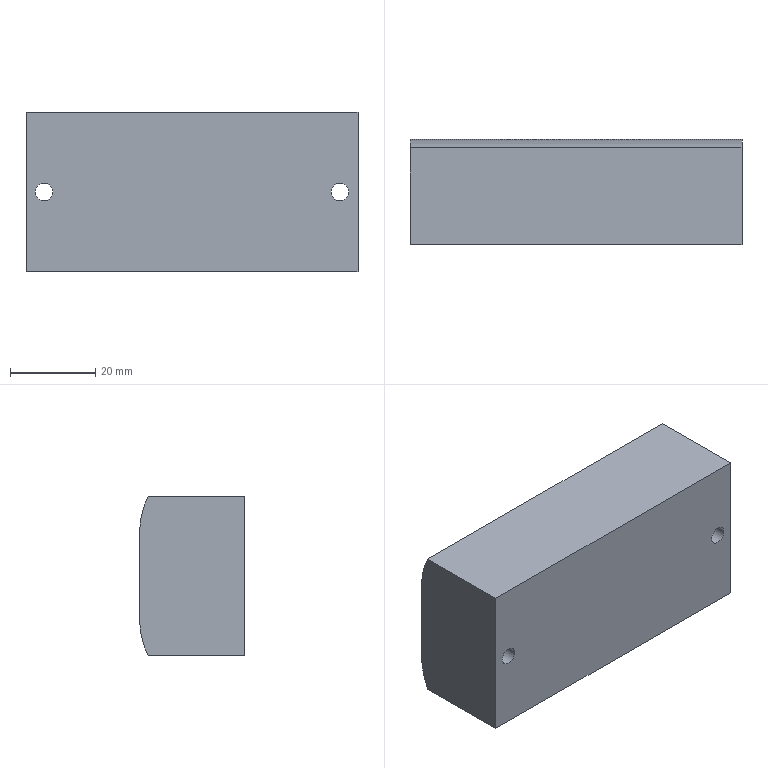Part | SolidWorks | features ICE 3, Extrusion 1 | 1 solid | 18 faces | box 77.96 x 24.63 x 37.4 mm | volume 70032 mm3 | cylinder 10 | plane 8 | commonest cylinder face diameters 4.1 x4 7 x4 40 x2
STEP:
#1=CARTESIAN_POINT('',(38.23,7.315,0.));
#2=VERTEX_POINT('',#1);
#3=CARTESIAN_POINT('',(31.23,7.315,0.));
#4=VERTEX_POINT('',#3);
#5=CARTESIAN_POINT('',(34.73,7.315,0.));
#6=DIRECTION('',(0.,1.,0.));
#7=DIRECTION('',(-1.,0.,0.));
#8=AXIS2_PLACEMENT_3D('',#5,#6,#7);
#9=CIRCLE('',#8,3.5);
#10=EDGE_CURVE('',#2,#4,#9,.T.);
#11=ORIENTED_EDGE('',*,*,#10,.F.);
#12=CARTESIAN_POINT('',(38.23,12.315,0.));
#13=VERTEX_POINT('',#12);
#14=CARTESIAN_POINT('',(38.23,7.315,0.));
#15=DIRECTION('',(0.,1.,0.));
#16=VECTOR('',#15,1000.);
#17=LINE('',#14,#16);
#18=EDGE_CURVE('',#2,#13,#17,.T.);
#19=ORIENTED_EDGE('',*,*,#18,.T.);
#20=CARTESIAN_POINT('',(31.23,12.315,0.));
#21=VERTEX_POINT('',#20);
#22=CARTESIAN_POINT('',(34.73,12.315,0.));
#23=DIRECTION('',(0.,1.,0.));
#24=DIRECTION('',(-1.,0.,0.));
#25=AXIS2_PLACEMENT_3D('',#22,#23,#24);
#26=CIRCLE('',#25,3.5);
#27=EDGE_CURVE('',#13,#21,#26,.T.);
#28=ORIENTED_EDGE('',*,*,#27,.T.);
#29=CARTESIAN_POINT('',(31.23,7.315,0.));
#30=DIRECTION('',(0.,1.,0.));
#31=VECTOR('',#30,1000.);
#32=LINE('',#29,#31);
#33=EDGE_CURVE('',#4,#21,#32,.T.);
#34=ORIENTED_EDGE('',*,*,#33,.F.);
#35=EDGE_LOOP('',(#11,#19,#28,#34));
#36=FACE_OUTER_BOUND('',#35,.T.);
#37=CARTESIAN_POINT('',(34.73,7.315,0.));
#38=DIRECTION('',(0.,1.,0.));
#39=DIRECTION('',(-1.,0.,0.));
#40=AXIS2_PLACEMENT_3D('',#37,#38,#39);
#41=CYLINDRICAL_SURFACE('',#40,3.5);
#42=ADVANCED_FACE('',(#36),#41,.F.);
#43=CARTESIAN_POINT('',(-31.23,7.315,0.));
#44=VERTEX_POINT('',#43);
#45=CARTESIAN_POINT('',(-38.23,7.315,0.));
#46=VERTEX_POINT('',#45);
#47=CARTESIAN_POINT('',(-34.73,7.315,0.));
#48=DIRECTION('',(0.,1.,0.));
#49=DIRECTION('',(-1.,0.,0.));
#50=AXIS2_PLACEMENT_3D('',#47,#48,#49);
#51=CIRCLE('',#50,3.5);
#52=EDGE_CURVE('',#44,#46,#51,.T.);
#53=ORIENTED_EDGE('',*,*,#52,.F.);
#54=CARTESIAN_POINT('',(-31.23,12.315,0.));
#55=VERTEX_POINT('',#54);
#56=CARTESIAN_POINT('',(-31.23,7.315,0.));
#57=DIRECTION('',(0.,1.,0.));
#58=VECTOR('',#57,1000.);
#59=LINE('',#56,#58);
#60=EDGE_CURVE('',#44,#55,#59,.T.);
#61=ORIENTED_EDGE('',*,*,#60,.T.);
#62=CARTESIAN_POINT('',(-38.23,12.315,0.));
#63=VERTEX_POINT('',#62);
#64=CARTESIAN_POINT('',(-34.73,12.315,0.));
#65=DIRECTION('',(0.,1.,0.));
#66=DIRECTION('',(-1.,0.,0.));
#67=AXIS2_PLACEMENT_3D('',#64,#65,#66);
#68=CIRCLE('',#67,3.5);
#69=EDGE_CURVE('',#55,#63,#68,.T.);
#70=ORIENTED_EDGE('',*,*,#69,.T.);
#71=CARTESIAN_POINT('',(-38.23,7.315,0.));
#72=DIRECTION('',(0.,1.,0.));
#73=VECTOR('',#72,1000.);
#74=LINE('',#71,#73);
#75=EDGE_CURVE('',#46,#63,#74,.T.);
#76=ORIENTED_EDGE('',*,*,#75,.F.);
#77=EDGE_LOOP('',(#53,#61,#70,#76));
#78=FACE_OUTER_BOUND('',#77,.T.);
#79=CARTESIAN_POINT('',(-34.73,7.315,0.));
#80=DIRECTION('',(0.,1.,0.));
#81=DIRECTION('',(-1.,0.,0.));
#82=AXIS2_PLACEMENT_3D('',#79,#80,#81);
#83=CYLINDRICAL_SURFACE('',#82,3.5);
#84=ADVANCED_FACE('',(#78),#83,.F.);
#85=CARTESIAN_POINT('',(-32.68,-12.315,0.));
#86=VERTEX_POINT('',#85);
#87=CARTESIAN_POINT('',(-36.78,-12.315,0.));
#88=VERTEX_POINT('',#87);
#89=CARTESIAN_POINT('',(-34.73,-12.315,0.));
#90=DIRECTION('',(0.,1.,0.));
#91=DIRECTION('',(-1.,0.,0.));
#92=AXIS2_PLACEMENT_3D('',#89,#90,#91);
#93=CIRCLE('',#92,2.05);
#94=EDGE_CURVE('',#86,#88,#93,.T.);
#95=ORIENTED_EDGE('',*,*,#94,.F.);
#96=CARTESIAN_POINT('',(-32.68,7.315,0.));
#97=VERTEX_POINT('',#96);
#98=CARTESIAN_POINT('',(-32.68,-12.315,0.));
#99=DIRECTION('',(0.,1.,0.));
#100=VECTOR('',#99,1000.);
#101=LINE('',#98,#100);
#102=EDGE_CURVE('',#86,#97,#101,.T.);
#103=ORIENTED_EDGE('',*,*,#102,.T.);
#104=CARTESIAN_POINT('',(-36.78,7.315,0.));
#105=VERTEX_POINT('',#104);
#106=CARTESIAN_POINT('',(-34.73,7.315,0.));
#107=DIRECTION('',(0.,-1.,0.));
#108=DIRECTION('',(-1.,0.,0.));
#109=AXIS2_PLACEMENT_3D('',#106,#107,#108);
#110=CIRCLE('',#109,2.05);
#111=EDGE_CURVE('',#105,#97,#110,.T.);
#112=ORIENTED_EDGE('',*,*,#111,.F.);
#113=CARTESIAN_POINT('',(-36.78,-12.315,0.));
#114=DIRECTION('',(0.,1.,0.));
#115=VECTOR('',#114,1000.);
#116=LINE('',#113,#115);
#117=EDGE_CURVE('',#88,#105,#116,.T.);
#118=ORIENTED_EDGE('',*,*,#117,.F.);
#119=EDGE_LOOP('',(#95,#103,#112,#118));
#120=FACE_OUTER_BOUND('',#119,.T.);
#121=CARTESIAN_POINT('',(-34.73,-12.315,0.));
#122=DIRECTION('',(0.,1.,0.));
#123=DIRECTION('',(-1.,0.,0.));
#124=AXIS2_PLACEMENT_3D('',#121,#122,#123);
#125=CYLINDRICAL_SURFACE('',#124,2.05);
#126=ADVANCED_FACE('',(#120),#125,.F.);
#127=CARTESIAN_POINT('',(36.78,-12.315,0.));
#128=VERTEX_POINT('',#127);
#129=CARTESIAN_POINT('',(32.68,-12.315,0.));
#130=VERTEX_POINT('',#129);
#131=CARTESIAN_POINT('',(34.73,-12.315,0.));
#132=DIRECTION('',(0.,1.,0.));
#133=DIRECTION('',(1.,0.,0.));
#134=AXIS2_PLACEMENT_3D('',#131,#132,#133);
#135=CIRCLE('',#134,2.05);
#136=EDGE_CURVE('',#128,#130,#135,.T.);
#137=ORIENTED_EDGE('',*,*,#136,.F.);
#138=CARTESIAN_POINT('',(36.78,7.315,0.));
#139=VERTEX_POINT('',#138);
#140=CARTESIAN_POINT('',(36.78,-12.315,0.));
#141=DIRECTION('',(0.,1.,0.));
#142=VECTOR('',#141,1000.);
#143=LINE('',#140,#142);
#144=EDGE_CURVE('',#128,#139,#143,.T.);
#145=ORIENTED_EDGE('',*,*,#144,.T.);
#146=CARTESIAN_POINT('',(32.68,7.315,0.));
#147=VERTEX_POINT('',#146);
#148=CARTESIAN_POINT('',(34.73,7.315,0.));
#149=DIRECTION('',(0.,-1.,0.));
#150=DIRECTION('',(-1.,0.,0.));
#151=AXIS2_PLACEMENT_3D('',#148,#149,#150);
#152=CIRCLE('',#151,2.05);
#153=EDGE_CURVE('',#147,#139,#152,.T.);
#154=ORIENTED_EDGE('',*,*,#153,.F.);
#155=CARTESIAN_POINT('',(32.68,-12.315,0.));
#156=DIRECTION('',(0.,1.,0.));
#157=VECTOR('',#156,1000.);
#158=LINE('',#155,#157);
#159=EDGE_CURVE('',#130,#147,#158,.T.);
#160=ORIENTED_EDGE('',*,*,#159,.F.);
#161=EDGE_LOOP('',(#137,#145,#154,#160));
#162=FACE_OUTER_BOUND('',#161,.T.);
#163=CARTESIAN_POINT('',(34.73,-12.315,0.));
#164=DIRECTION('',(0.,1.,0.));
#165=DIRECTION('',(-1.,0.,0.));
#166=AXIS2_PLACEMENT_3D('',#163,#164,#165);
#167=CYLINDRICAL_SURFACE('',#166,2.05);
#168=ADVANCED_FACE('',(#162),#167,.F.);
#169=ORIENTED_EDGE('',*,*,#144,.F.);
#170=CARTESIAN_POINT('',(34.73,-12.315,0.));
#171=DIRECTION('',(0.,1.,0.));
#172=DIRECTION('',(1.,0.,0.));
#173=AXIS2_PLACEMENT_3D('',#170,#171,#172);
#174=CIRCLE('',#173,2.05);
#175=EDGE_CURVE('',#130,#128,#174,.T.);
#176=ORIENTED_EDGE('',*,*,#175,.F.);
#177=ORIENTED_EDGE('',*,*,#159,.T.);
#178=CARTESIAN_POINT('',(34.73,7.315,0.));
#179=DIRECTION('',(0.,-1.,0.));
#180=DIRECTION('',(-1.,0.,0.));
#181=AXIS2_PLACEMENT_3D('',#178,#179,#180);
#182=CIRCLE('',#181,2.05);
#183=EDGE_CURVE('',#139,#147,#182,.T.);
#184=ORIENTED_EDGE('',*,*,#183,.F.);
#185=EDGE_LOOP('',(#169,#176,#177,#184));
#186=FACE_OUTER_BOUND('',#185,.T.);
#187=CARTESIAN_POINT('',(34.73,-12.315,0.));
#188=DIRECTION('',(0.,1.,0.));
#189=DIRECTION('',(-1.,0.,0.));
#190=AXIS2_PLACEMENT_3D('',#187,#188,#189);
#191=CYLINDRICAL_SURFACE('',#190,2.05);
#192=ADVANCED_FACE('',(#186),#191,.F.);
#193=ORIENTED_EDGE('',*,*,#102,.F.);
#194=CARTESIAN_POINT('',(-34.73,-12.315,0.));
#195=DIRECTION('',(0.,1.,0.));
#196=DIRECTION('',(-1.,0.,0.));
#197=AXIS2_PLACEMENT_3D('',#194,#195,#196);
#198=CIRCLE('',#197,2.05);
#199=EDGE_CURVE('',#88,#86,#198,.T.);
#200=ORIENTED_EDGE('',*,*,#199,.F.);
#201=ORIENTED_EDGE('',*,*,#117,.T.);
#202=CARTESIAN_POINT('',(-34.73,7.315,0.));
#203=DIRECTION('',(0.,-1.,0.));
#204=DIRECTION('',(-1.,0.,0.));
#205=AXIS2_PLACEMENT_3D('',#202,#203,#204);
#206=CIRCLE('',#205,2.05);
#207=EDGE_CURVE('',#97,#105,#206,.T.);
#208=ORIENTED_EDGE('',*,*,#207,.F.);
#209=EDGE_LOOP('',(#193,#200,#201,#208));
#210=FACE_OUTER_BOUND('',#209,.T.);
#211=CARTESIAN_POINT('',(-34.73,-12.315,0.));
#212=DIRECTION('',(0.,1.,0.));
#213=DIRECTION('',(-1.,0.,0.));
#214=AXIS2_PLACEMENT_3D('',#211,#212,#213);
#215=CYLINDRICAL_SURFACE('',#214,2.05);
#216=ADVANCED_FACE('',(#210),#215,.F.);
#217=CARTESIAN_POINT('',(-38.98,10.315,18.7));
#218=VERTEX_POINT('',#217);
#219=CARTESIAN_POINT('',(-38.98,-12.315,18.7));
#220=VERTEX_POINT('',#219);
#221=CARTESIAN_POINT('',(-38.98,12.315,18.7));
#222=DIRECTION('',(0.,-1.,0.));
#223=VECTOR('',#222,1000.);
#224=LINE('',#221,#223);
#225=EDGE_CURVE('',#218,#220,#224,.T.);
#226=ORIENTED_EDGE('',*,*,#225,.F.);
#227=CARTESIAN_POINT('',(-38.98,12.315,10.7));
#228=VERTEX_POINT('',#227);
#229=CARTESIAN_POINT('',(-38.98,-7.671,9.953));
#230=DIRECTION('',(-1.,0.,0.));
#231=DIRECTION('',(0.,1.,0.));
#232=AXIS2_PLACEMENT_3D('',#229,#230,#231);
#233=CIRCLE('',#232,20.);
#234=EDGE_CURVE('',#218,#228,#233,.T.);
#235=ORIENTED_EDGE('',*,*,#234,.T.);
#236=CARTESIAN_POINT('',(-38.98,12.315,-10.7));
#237=VERTEX_POINT('',#236);
#238=CARTESIAN_POINT('',(-38.98,12.315,18.7));
#239=DIRECTION('',(0.,0.,-1.));
#240=VECTOR('',#239,1000.);
#241=LINE('',#238,#240);
#242=EDGE_CURVE('',#228,#237,#241,.T.);
#243=ORIENTED_EDGE('',*,*,#242,.T.);
#244=CARTESIAN_POINT('',(-38.98,10.315,-18.7));
#245=VERTEX_POINT('',#244);
#246=CARTESIAN_POINT('',(-38.98,-7.671,-9.953));
#247=DIRECTION('',(-1.,0.,0.));
#248=DIRECTION('',(0.,-1.,0.));
#249=AXIS2_PLACEMENT_3D('',#246,#247,#248);
#250=CIRCLE('',#249,20.);
#251=EDGE_CURVE('',#237,#245,#250,.T.);
#252=ORIENTED_EDGE('',*,*,#251,.T.);
#253=CARTESIAN_POINT('',(-38.98,-12.315,-18.7));
#254=VERTEX_POINT('',#253);
#255=CARTESIAN_POINT('',(-38.98,12.315,-18.7));
#256=DIRECTION('',(0.,-1.,0.));
#257=VECTOR('',#256,1000.);
#258=LINE('',#255,#257);
#259=EDGE_CURVE('',#245,#254,#258,.T.);
#260=ORIENTED_EDGE('',*,*,#259,.T.);
#261=CARTESIAN_POINT('',(-38.98,-12.315,18.7));
#262=DIRECTION('',(0.,0.,-1.));
#263=VECTOR('',#262,1000.);
#264=LINE('',#261,#263);
#265=EDGE_CURVE('',#220,#254,#264,.T.);
#266=ORIENTED_EDGE('',*,*,#265,.F.);
#267=EDGE_LOOP('',(#226,#235,#243,#252,#260,#266));
#268=FACE_OUTER_BOUND('',#267,.T.);
#269=CARTESIAN_POINT('',(-38.98,12.315,18.7));
#270=DIRECTION('',(1.,0.,0.));
#271=DIRECTION('',(0.,0.,-1.));
#272=AXIS2_PLACEMENT_3D('',#269,#270,#271);
#273=PLANE('',#272);
#274=ADVANCED_FACE('',(#268),#273,.F.);
#275=ORIENTED_EDGE('',*,*,#199,.T.);
#276=ORIENTED_EDGE('',*,*,#94,.T.);
#277=EDGE_LOOP('',(#275,#276));
#278=FACE_BOUND('',#277,.T.);
#279=ORIENTED_EDGE('',*,*,#175,.T.);
#280=ORIENTED_EDGE('',*,*,#136,.T.);
#281=EDGE_LOOP('',(#279,#280));
#282=FACE_BOUND('',#281,.T.);
#283=CARTESIAN_POINT('',(38.98,-12.315,-18.7));
#284=VERTEX_POINT('',#283);
#285=CARTESIAN_POINT('',(-38.98,-12.315,-18.7));
#286=DIRECTION('',(1.,0.,0.));
#287=VECTOR('',#286,1000.);
#288=LINE('',#285,#287);
#289=EDGE_CURVE('',#254,#284,#288,.T.);
#290=ORIENTED_EDGE('',*,*,#289,.T.);
#291=CARTESIAN_POINT('',(38.98,-12.315,18.7));
#292=VERTEX_POINT('',#291);
#293=CARTESIAN_POINT('',(38.98,-12.315,18.7));
#294=DIRECTION('',(0.,0.,-1.));
#295=VECTOR('',#294,1000.);
#296=LINE('',#293,#295);
#297=EDGE_CURVE('',#292,#284,#296,.T.);
#298=ORIENTED_EDGE('',*,*,#297,.F.);
#299=CARTESIAN_POINT('',(-38.98,-12.315,18.7));
#300=DIRECTION('',(1.,0.,0.));
#301=VECTOR('',#300,1000.);
#302=LINE('',#299,#301);
#303=EDGE_CURVE('',#220,#292,#302,.T.);
#304=ORIENTED_EDGE('',*,*,#303,.F.);
#305=ORIENTED_EDGE('',*,*,#265,.T.);
#306=EDGE_LOOP('',(#290,#298,#304,#305));
#307=FACE_OUTER_BOUND('',#306,.T.);
#308=CARTESIAN_POINT('',(-38.98,-12.315,18.7));
#309=DIRECTION('',(0.,1.,0.));
#310=DIRECTION('',(-1.,0.,0.));
#311=AXIS2_PLACEMENT_3D('',#308,#309,#310);
#312=PLANE('',#311);
#313=ADVANCED_FACE('',(#278,#282,#307),#312,.F.);
#314=CARTESIAN_POINT('',(38.98,12.315,10.7));
#315=VERTEX_POINT('',#314);
#316=CARTESIAN_POINT('',(38.98,12.315,-10.7));
#317=VERTEX_POINT('',#316);
#318=CARTESIAN_POINT('',(38.98,12.315,18.7));
#319=DIRECTION('',(0.,0.,-1.));
#320=VECTOR('',#319,1000.);
#321=LINE('',#318,#320);
#322=EDGE_CURVE('',#315,#317,#321,.T.);
#323=ORIENTED_EDGE('',*,*,#322,.F.);
#324=CARTESIAN_POINT('',(38.98,10.315,18.7));
#325=VERTEX_POINT('',#324);
#326=CARTESIAN_POINT('',(38.98,-7.671,9.953));
#327=DIRECTION('',(-1.,0.,0.));
#328=DIRECTION('',(0.,1.,0.));
#329=AXIS2_PLACEMENT_3D('',#326,#327,#328);
#330=CIRCLE('',#329,20.);
#331=EDGE_CURVE('',#325,#315,#330,.T.);
#332=ORIENTED_EDGE('',*,*,#331,.F.);
#333=CARTESIAN_POINT('',(38.98,12.315,18.7));
#334=DIRECTION('',(0.,1.,0.));
#335=VECTOR('',#334,1000.);
#336=LINE('',#333,#335);
#337=EDGE_CURVE('',#292,#325,#336,.T.);
#338=ORIENTED_EDGE('',*,*,#337,.F.);
#339=ORIENTED_EDGE('',*,*,#297,.T.);
#340=CARTESIAN_POINT('',(38.98,10.315,-18.7));
#341=VERTEX_POINT('',#340);
#342=CARTESIAN_POINT('',(38.98,12.315,-18.7));
#343=DIRECTION('',(0.,1.,0.));
#344=VECTOR('',#343,1000.);
#345=LINE('',#342,#344);
#346=EDGE_CURVE('',#284,#341,#345,.T.);
#347=ORIENTED_EDGE('',*,*,#346,.T.);
#348=CARTESIAN_POINT('',(38.98,-7.671,-9.953));
#349=DIRECTION('',(-1.,0.,0.));
#350=DIRECTION('',(0.,-1.,0.));
#351=AXIS2_PLACEMENT_3D('',#348,#349,#350);
#352=CIRCLE('',#351,20.);
#353=EDGE_CURVE('',#317,#341,#352,.T.);
#354=ORIENTED_EDGE('',*,*,#353,.F.);
#355=EDGE_LOOP('',(#323,#332,#338,#339,#347,#354));
#356=FACE_OUTER_BOUND('',#355,.T.);
#357=CARTESIAN_POINT('',(38.98,12.315,18.7));
#358=DIRECTION('',(-1.,0.,0.));
#359=DIRECTION('',(0.,0.,1.));
#360=AXIS2_PLACEMENT_3D('',#357,#358,#359);
#361=PLANE('',#360);
#362=ADVANCED_FACE('',(#356),#361,.F.);
#363=CARTESIAN_POINT('',(-34.73,12.315,0.));
#364=DIRECTION('',(0.,1.,0.));
#365=DIRECTION('',(-1.,0.,0.));
#366=AXIS2_PLACEMENT_3D('',#363,#364,#365);
#367=CIRCLE('',#366,3.5);
#368=EDGE_CURVE('',#63,#55,#367,.T.);
#369=ORIENTED_EDGE('',*,*,#368,.F.);
#370=ORIENTED_EDGE('',*,*,#69,.F.);
#371=EDGE_LOOP('',(#369,#370));
#372=FACE_BOUND('',#371,.T.);
#373=CARTESIAN_POINT('',(34.73,12.315,0.));
#374=DIRECTION('',(0.,1.,0.));
#375=DIRECTION('',(-1.,0.,0.));
#376=AXIS2_PLACEMENT_3D('',#373,#374,#375);
#377=CIRCLE('',#376,3.5);
#378=EDGE_CURVE('',#21,#13,#377,.T.);
#379=ORIENTED_EDGE('',*,*,#378,.F.);
#380=ORIENTED_EDGE('',*,*,#27,.F.);
#381=EDGE_LOOP('',(#379,#380));
#382=FACE_BOUND('',#381,.T.);
#383=ORIENTED_EDGE('',*,*,#242,.F.);
#384=CARTESIAN_POINT('',(-38.98,12.315,10.7));
#385=DIRECTION('',(1.,0.,0.));
#386=VECTOR('',#385,1000.);
#387=LINE('',#384,#386);
#388=EDGE_CURVE('',#228,#315,#387,.T.);
#389=ORIENTED_EDGE('',*,*,#388,.T.);
#390=ORIENTED_EDGE('',*,*,#322,.T.);
#391=CARTESIAN_POINT('',(-38.98,12.315,-10.7));
#392=DIRECTION('',(1.,0.,0.));
#393=VECTOR('',#392,1000.);
#394=LINE('',#391,#393);
#395=EDGE_CURVE('',#237,#317,#394,.T.);
#396=ORIENTED_EDGE('',*,*,#395,.F.);
#397=EDGE_LOOP('',(#383,#389,#390,#396));
#398=FACE_OUTER_BOUND('',#397,.T.);
#399=CARTESIAN_POINT('',(-38.98,12.315,18.7));
#400=DIRECTION('',(0.,-1.,0.));
#401=DIRECTION('',(1.,0.,0.));
#402=AXIS2_PLACEMENT_3D('',#399,#400,#401);
#403=PLANE('',#402);
#404=ADVANCED_FACE('',(#372,#382,#398),#403,.F.);
#405=CARTESIAN_POINT('',(-38.98,10.315,18.7));
#406=DIRECTION('',(1.,0.,0.));
#407=VECTOR('',#406,1000.);
#408=LINE('',#405,#407);
#409=EDGE_CURVE('',#218,#325,#408,.T.);
#410=ORIENTED_EDGE('',*,*,#409,.F.);
#411=ORIENTED_EDGE('',*,*,#225,.T.);
#412=ORIENTED_EDGE('',*,*,#303,.T.);
#413=ORIENTED_EDGE('',*,*,#337,.T.);
#414=EDGE_LOOP('',(#410,#411,#412,#413));
#415=FACE_OUTER_BOUND('',#414,.T.);
#416=CARTESIAN_POINT('',(0.,0.,18.7));
#417=DIRECTION('',(0.,0.,1.));
#418=DIRECTION('',(1.,0.,0.));
#419=AXIS2_PLACEMENT_3D('',#416,#417,#418);
#420=PLANE('',#419);
#421=ADVANCED_FACE('',(#415),#420,.T.);
#422=ORIENTED_EDGE('',*,*,#259,.F.);
#423=CARTESIAN_POINT('',(-38.98,10.315,-18.7));
#424=DIRECTION('',(1.,0.,0.));
#425=VECTOR('',#424,1000.);
#426=LINE('',#423,#425);
#427=EDGE_CURVE('',#245,#341,#426,.T.);
#428=ORIENTED_EDGE('',*,*,#427,.T.);
#429=ORIENTED_EDGE('',*,*,#346,.F.);
#430=ORIENTED_EDGE('',*,*,#289,.F.);
#431=EDGE_LOOP('',(#422,#428,#429,#430));
#432=FACE_OUTER_BOUND('',#431,.T.);
#433=CARTESIAN_POINT('',(0.,0.,-18.7));
#434=DIRECTION('',(0.,0.,1.));
#435=DIRECTION('',(1.,0.,0.));
#436=AXIS2_PLACEMENT_3D('',#433,#434,#435);
#437=PLANE('',#436);
#438=ADVANCED_FACE('',(#432),#437,.F.);
#439=ORIENTED_EDGE('',*,*,#353,.T.);
#440=ORIENTED_EDGE('',*,*,#427,.F.);
#441=ORIENTED_EDGE('',*,*,#251,.F.);
#442=ORIENTED_EDGE('',*,*,#395,.T.);
#443=EDGE_LOOP('',(#439,#440,#441,#442));
#444=FACE_OUTER_BOUND('',#443,.T.);
#445=CARTESIAN_POINT('',(-38.98,-7.671,-9.953));
#446=DIRECTION('',(1.,0.,0.));
#447=DIRECTION('',(0.,1.,0.));
#448=AXIS2_PLACEMENT_3D('',#445,#446,#447);
#449=CYLINDRICAL_SURFACE('',#448,20.);
#450=ADVANCED_FACE('',(#444),#449,.T.);
#451=ORIENTED_EDGE('',*,*,#331,.T.);
#452=ORIENTED_EDGE('',*,*,#388,.F.);
#453=ORIENTED_EDGE('',*,*,#234,.F.);
#454=ORIENTED_EDGE('',*,*,#409,.T.);
#455=EDGE_LOOP('',(#451,#452,#453,#454));
#456=FACE_OUTER_BOUND('',#455,.T.);
#457=CARTESIAN_POINT('',(-38.98,-7.671,9.953));
#458=DIRECTION('',(1.,0.,0.));
#459=DIRECTION('',(0.,1.,0.));
#460=AXIS2_PLACEMENT_3D('',#457,#458,#459);
#461=CYLINDRICAL_SURFACE('',#460,20.);
#462=ADVANCED_FACE('',(#456),#461,.T.);
#463=CARTESIAN_POINT('',(-34.73,7.315,0.));
#464=DIRECTION('',(0.,1.,0.));
#465=DIRECTION('',(-1.,0.,0.));
#466=AXIS2_PLACEMENT_3D('',#463,#464,#465);
#467=CIRCLE('',#466,3.5);
#468=EDGE_CURVE('',#46,#44,#467,.T.);
#469=ORIENTED_EDGE('',*,*,#468,.T.);
#470=ORIENTED_EDGE('',*,*,#52,.T.);
#471=EDGE_LOOP('',(#469,#470));
#472=FACE_OUTER_BOUND('',#471,.T.);
#473=ORIENTED_EDGE('',*,*,#111,.T.);
#474=ORIENTED_EDGE('',*,*,#207,.T.);
#475=EDGE_LOOP('',(#473,#474));
#476=FACE_BOUND('',#475,.T.);
#477=CARTESIAN_POINT('',(-34.73,7.315,0.));
#478=DIRECTION('',(0.,1.,0.));
#479=DIRECTION('',(-1.,0.,0.));
#480=AXIS2_PLACEMENT_3D('',#477,#478,#479);
#481=PLANE('',#480);
#482=ADVANCED_FACE('',(#472,#476),#481,.T.);
#483=ORIENTED_EDGE('',*,*,#60,.F.);
#484=ORIENTED_EDGE('',*,*,#468,.F.);
#485=ORIENTED_EDGE('',*,*,#75,.T.);
#486=ORIENTED_EDGE('',*,*,#368,.T.);
#487=EDGE_LOOP('',(#483,#484,#485,#486));
#488=FACE_OUTER_BOUND('',#487,.T.);
#489=CARTESIAN_POINT('',(-34.73,7.315,0.));
#490=DIRECTION('',(0.,1.,0.));
#491=DIRECTION('',(-1.,0.,0.));
#492=AXIS2_PLACEMENT_3D('',#489,#490,#491);
#493=CYLINDRICAL_SURFACE('',#492,3.5);
#494=ADVANCED_FACE('',(#488),#493,.F.);
#495=CARTESIAN_POINT('',(34.73,7.315,0.));
#496=DIRECTION('',(0.,1.,0.));
#497=DIRECTION('',(-1.,0.,0.));
#498=AXIS2_PLACEMENT_3D('',#495,#496,#497);
#499=CIRCLE('',#498,3.5);
#500=EDGE_CURVE('',#4,#2,#499,.T.);
#501=ORIENTED_EDGE('',*,*,#500,.T.);
#502=ORIENTED_EDGE('',*,*,#10,.T.);
#503=EDGE_LOOP('',(#501,#502));
#504=FACE_OUTER_BOUND('',#503,.T.);
#505=ORIENTED_EDGE('',*,*,#153,.T.);
#506=ORIENTED_EDGE('',*,*,#183,.T.);
#507=EDGE_LOOP('',(#505,#506));
#508=FACE_BOUND('',#507,.T.);
#509=CARTESIAN_POINT('',(34.73,7.315,0.));
#510=DIRECTION('',(0.,1.,0.));
#511=DIRECTION('',(-1.,0.,0.));
#512=AXIS2_PLACEMENT_3D('',#509,#510,#511);
#513=PLANE('',#512);
#514=ADVANCED_FACE('',(#504,#508),#513,.T.);
#515=ORIENTED_EDGE('',*,*,#18,.F.);
#516=ORIENTED_EDGE('',*,*,#500,.F.);
#517=ORIENTED_EDGE('',*,*,#33,.T.);
#518=ORIENTED_EDGE('',*,*,#378,.T.);
#519=EDGE_LOOP('',(#515,#516,#517,#518));
#520=FACE_OUTER_BOUND('',#519,.T.);
#521=CARTESIAN_POINT('',(34.73,7.315,0.));
#522=DIRECTION('',(0.,1.,0.));
#523=DIRECTION('',(-1.,0.,0.));
#524=AXIS2_PLACEMENT_3D('',#521,#522,#523);
#525=CYLINDRICAL_SURFACE('',#524,3.5);
#526=ADVANCED_FACE('',(#520),#525,.F.);
#527=CLOSED_SHELL('',(#42,#84,#126,#168,#192,#216,#274,#313,#362,#404,#421,#438,#450,#462,#482,#494,#514,#526));
#528=MANIFOLD_SOLID_BREP('',#527);
#529=CARTESIAN_POINT('',(0.,0.,0.));
#530=DIRECTION('',(0.,0.,1.));
#531=DIRECTION('',(1.,0.,0.));
#532=AXIS2_PLACEMENT_3D('',#529,#530,#531);
#533=(LENGTH_UNIT()NAMED_UNIT(*)SI_UNIT(.MILLI.,.METRE.));
#534=UNCERTAINTY_MEASURE_WITH_UNIT(LENGTH_MEASURE(0.00001),#533,'','');
#535=(NAMED_UNIT(*)PLANE_ANGLE_UNIT()SI_UNIT($,.RADIAN.));
#536=(NAMED_UNIT(*)SI_UNIT($,.STERADIAN.)SOLID_ANGLE_UNIT());
#537=(GEOMETRIC_REPRESENTATION_CONTEXT(3)GLOBAL_UNCERTAINTY_ASSIGNED_CONTEXT((#534))GLOBAL_UNIT_ASSIGNED_CONTEXT((#533,#535,#536))REPRESENTATION_CONTEXT('',''));
#538=ADVANCED_BREP_SHAPE_REPRESENTATION('',(#528,#532),#537);